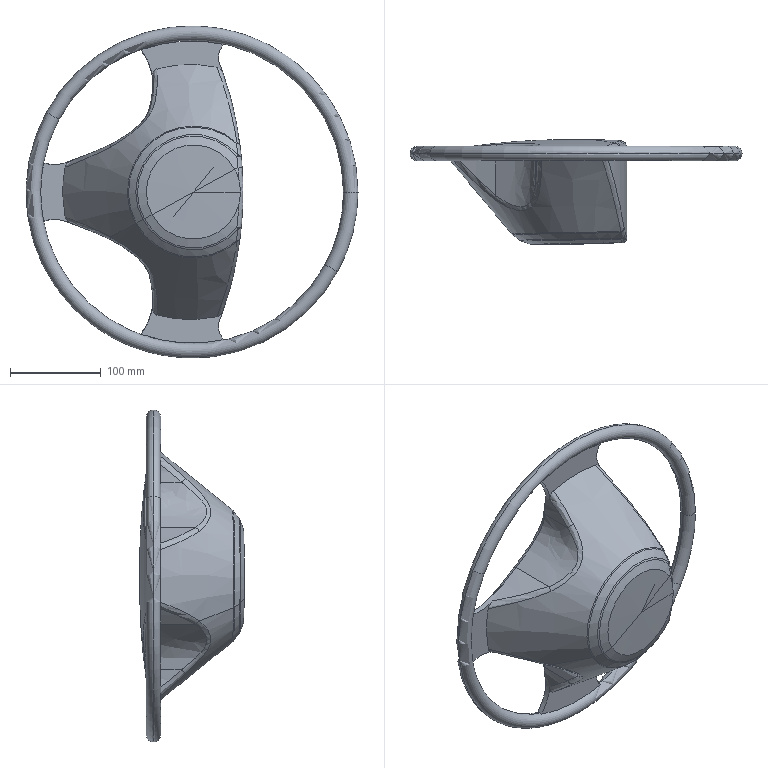Part | SolidWorks | features MBimport 1 | 2 solids | 72 faces | box 366 x 115.12 x 366 mm | volume 3175003 mm3 | spline 26 | cone 14 | torus 13 | cylinder 9 | plane 6 | sphere 4 | commonest cylinder face diameters 38.503 x4 333.031 x4 800 x1